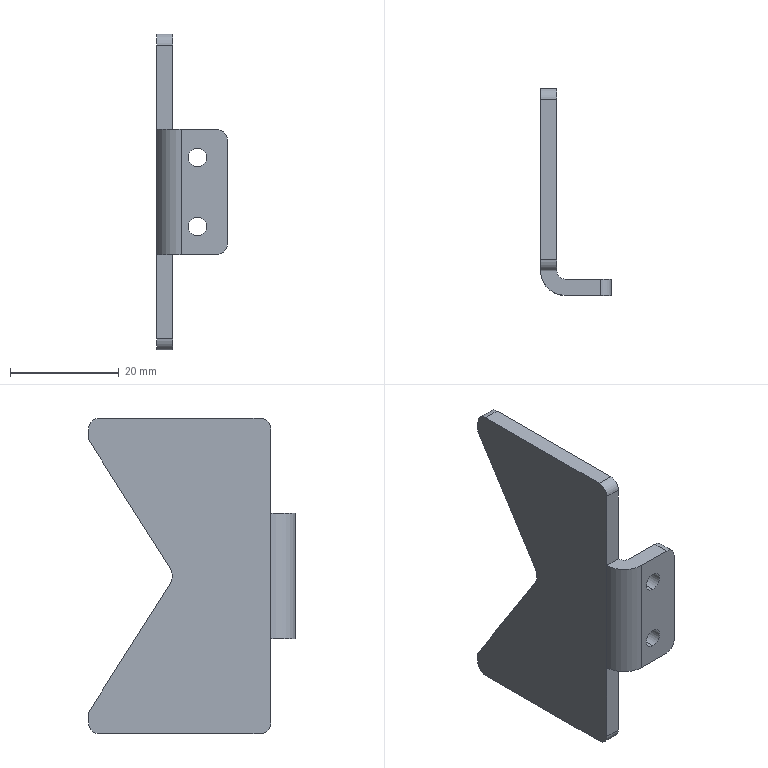Part | SolidWorks | features Fillet 2, ICE 2, FlatPattern 1, HoleWzd 1, SMBaseFlange 1, SheetMetal 1 | 1 solid | 29 faces | box 13 x 38 x 58 mm | volume 5478 mm3 | plane 16 | cylinder 13 | commonest cylinder face diameters 4 x6 3.4 x4 3 x1 6 x1 9 x1
STEP:
#1=CARTESIAN_POINT('',(4.5,-3.,-8.05));
#2=VERTEX_POINT('',#1);
#3=CARTESIAN_POINT('',(4.5,-3.,-4.65));
#4=VERTEX_POINT('',#3);
#5=CARTESIAN_POINT('',(4.5,-3.,-6.35));
#6=DIRECTION('',(0.,1.,0.));
#7=DIRECTION('',(0.,0.,1.));
#8=AXIS2_PLACEMENT_3D('',#5,#6,#7);
#9=CIRCLE('',#8,1.7);
#10=EDGE_CURVE('',#2,#4,#9,.T.);
#11=ORIENTED_EDGE('',*,*,#10,.F.);
#12=CARTESIAN_POINT('',(4.5,0.,-8.05));
#13=VERTEX_POINT('',#12);
#14=CARTESIAN_POINT('',(4.5,0.,-8.05));
#15=DIRECTION('',(0.,1.,0.));
#16=VECTOR('',#15,1000.);
#17=LINE('',#14,#16);
#18=EDGE_CURVE('',#2,#13,#17,.T.);
#19=ORIENTED_EDGE('',*,*,#18,.T.);
#20=CARTESIAN_POINT('',(4.5,0.,-4.65));
#21=VERTEX_POINT('',#20);
#22=CARTESIAN_POINT('',(4.5,0.,-6.35));
#23=DIRECTION('',(0.,1.,0.));
#24=DIRECTION('',(0.,0.,1.));
#25=AXIS2_PLACEMENT_3D('',#22,#23,#24);
#26=CIRCLE('',#25,1.7);
#27=EDGE_CURVE('',#13,#21,#26,.T.);
#28=ORIENTED_EDGE('',*,*,#27,.T.);
#29=CARTESIAN_POINT('',(4.5,0.,-4.65));
#30=DIRECTION('',(0.,1.,0.));
#31=VECTOR('',#30,1000.);
#32=LINE('',#29,#31);
#33=EDGE_CURVE('',#4,#21,#32,.T.);
#34=ORIENTED_EDGE('',*,*,#33,.F.);
#35=EDGE_LOOP('',(#11,#19,#28,#34));
#36=FACE_OUTER_BOUND('',#35,.T.);
#37=CARTESIAN_POINT('',(4.5,0.,-6.35));
#38=DIRECTION('',(0.,1.,0.));
#39=DIRECTION('',(0.,0.,1.));
#40=AXIS2_PLACEMENT_3D('',#37,#38,#39);
#41=CYLINDRICAL_SURFACE('',#40,1.7);
#42=ADVANCED_FACE('',(#36),#41,.F.);
#43=CARTESIAN_POINT('',(4.5,-3.,4.65));
#44=VERTEX_POINT('',#43);
#45=CARTESIAN_POINT('',(4.5,-3.,8.05));
#46=VERTEX_POINT('',#45);
#47=CARTESIAN_POINT('',(4.5,-3.,6.35));
#48=DIRECTION('',(0.,1.,0.));
#49=DIRECTION('',(0.,0.,1.));
#50=AXIS2_PLACEMENT_3D('',#47,#48,#49);
#51=CIRCLE('',#50,1.7);
#52=EDGE_CURVE('',#44,#46,#51,.T.);
#53=ORIENTED_EDGE('',*,*,#52,.F.);
#54=CARTESIAN_POINT('',(4.5,0.,4.65));
#55=VERTEX_POINT('',#54);
#56=CARTESIAN_POINT('',(4.5,0.,4.65));
#57=DIRECTION('',(0.,1.,0.));
#58=VECTOR('',#57,1000.);
#59=LINE('',#56,#58);
#60=EDGE_CURVE('',#44,#55,#59,.T.);
#61=ORIENTED_EDGE('',*,*,#60,.T.);
#62=CARTESIAN_POINT('',(4.5,0.,8.05));
#63=VERTEX_POINT('',#62);
#64=CARTESIAN_POINT('',(4.5,0.,6.35));
#65=DIRECTION('',(0.,1.,0.));
#66=DIRECTION('',(0.,0.,1.));
#67=AXIS2_PLACEMENT_3D('',#64,#65,#66);
#68=CIRCLE('',#67,1.7);
#69=EDGE_CURVE('',#55,#63,#68,.T.);
#70=ORIENTED_EDGE('',*,*,#69,.T.);
#71=CARTESIAN_POINT('',(4.5,0.,8.05));
#72=DIRECTION('',(0.,1.,0.));
#73=VECTOR('',#72,1000.);
#74=LINE('',#71,#73);
#75=EDGE_CURVE('',#46,#63,#74,.T.);
#76=ORIENTED_EDGE('',*,*,#75,.F.);
#77=EDGE_LOOP('',(#53,#61,#70,#76));
#78=FACE_OUTER_BOUND('',#77,.T.);
#79=CARTESIAN_POINT('',(4.5,0.,6.35));
#80=DIRECTION('',(0.,1.,0.));
#81=DIRECTION('',(0.,0.,1.));
#82=AXIS2_PLACEMENT_3D('',#79,#80,#81);
#83=CYLINDRICAL_SURFACE('',#82,1.7);
#84=ADVANCED_FACE('',(#78),#83,.F.);
#85=CARTESIAN_POINT('',(8.,0.,-11.5));
#86=VERTEX_POINT('',#85);
#87=CARTESIAN_POINT('',(1.5,0.,-11.5));
#88=VERTEX_POINT('',#87);
#89=CARTESIAN_POINT('',(0.,0.,-11.5));
#90=DIRECTION('',(-1.,0.,0.));
#91=VECTOR('',#90,1000.);
#92=LINE('',#89,#91);
#93=EDGE_CURVE('',#86,#88,#92,.T.);
#94=ORIENTED_EDGE('',*,*,#93,.F.);
#95=CARTESIAN_POINT('',(8.,-3.,-11.5));
#96=VERTEX_POINT('',#95);
#97=CARTESIAN_POINT('',(8.,1.5,-11.5));
#98=DIRECTION('',(0.,-1.,0.));
#99=VECTOR('',#98,1000.);
#100=LINE('',#97,#99);
#101=EDGE_CURVE('',#86,#96,#100,.T.);
#102=ORIENTED_EDGE('',*,*,#101,.T.);
#103=CARTESIAN_POINT('',(1.5,-3.,-11.5));
#104=VERTEX_POINT('',#103);
#105=CARTESIAN_POINT('',(-3.,-3.,-11.5));
#106=DIRECTION('',(1.,0.,0.));
#107=VECTOR('',#106,1000.);
#108=LINE('',#105,#107);
#109=EDGE_CURVE('',#104,#96,#108,.T.);
#110=ORIENTED_EDGE('',*,*,#109,.F.);
#111=CARTESIAN_POINT('',(1.5,-3.,-11.5));
#112=DIRECTION('',(0.,1.,0.));
#113=VECTOR('',#112,1000.);
#114=LINE('',#111,#113);
#115=EDGE_CURVE('',#104,#88,#114,.T.);
#116=ORIENTED_EDGE('',*,*,#115,.T.);
#117=EDGE_LOOP('',(#94,#102,#110,#116));
#118=FACE_OUTER_BOUND('',#117,.T.);
#119=CARTESIAN_POINT('',(-3.,1.5,-11.5));
#120=DIRECTION('',(0.,0.,1.));
#121=DIRECTION('',(0.,-1.,0.));
#122=AXIS2_PLACEMENT_3D('',#119,#120,#121);
#123=PLANE('',#122);
#124=ADVANCED_FACE('',(#118),#123,.F.);
#125=CARTESIAN_POINT('',(-3.,35.,-27.));
#126=VERTEX_POINT('',#125);
#127=CARTESIAN_POINT('',(-3.,35.,-25.));
#128=VERTEX_POINT('',#127);
#129=CARTESIAN_POINT('',(-3.,35.,-29.));
#130=DIRECTION('',(0.,0.,1.));
#131=VECTOR('',#130,1000.);
#132=LINE('',#129,#131);
#133=EDGE_CURVE('',#126,#128,#132,.T.);
#134=ORIENTED_EDGE('',*,*,#133,.T.);
#135=CARTESIAN_POINT('',(0.,35.,-25.));
#136=VERTEX_POINT('',#135);
#137=CARTESIAN_POINT('',(-3.,35.,-25.));
#138=DIRECTION('',(1.,0.,0.));
#139=VECTOR('',#138,1000.);
#140=LINE('',#137,#139);
#141=EDGE_CURVE('',#128,#136,#140,.T.);
#142=ORIENTED_EDGE('',*,*,#141,.T.);
#143=CARTESIAN_POINT('',(0.,35.,-27.));
#144=VERTEX_POINT('',#143);
#145=CARTESIAN_POINT('',(0.,35.,-29.));
#146=DIRECTION('',(0.,0.,1.));
#147=VECTOR('',#146,1000.);
#148=LINE('',#145,#147);
#149=EDGE_CURVE('',#144,#136,#148,.T.);
#150=ORIENTED_EDGE('',*,*,#149,.F.);
#151=CARTESIAN_POINT('',(-3.,35.,-27.));
#152=DIRECTION('',(-1.,0.,0.));
#153=VECTOR('',#152,1000.);
#154=LINE('',#151,#153);
#155=EDGE_CURVE('',#144,#126,#154,.T.);
#156=ORIENTED_EDGE('',*,*,#155,.T.);
#157=EDGE_LOOP('',(#134,#142,#150,#156));
#158=FACE_OUTER_BOUND('',#157,.T.);
#159=CARTESIAN_POINT('',(-3.,35.,-29.));
#160=DIRECTION('',(0.,-1.,0.));
#161=DIRECTION('',(0.,0.,-1.));
#162=AXIS2_PLACEMENT_3D('',#159,#160,#161);
#163=PLANE('',#162);
#164=ADVANCED_FACE('',(#158),#163,.F.);
#165=CARTESIAN_POINT('',(0.,33.,-29.));
#166=VERTEX_POINT('',#165);
#167=CARTESIAN_POINT('',(0.,3.5,-29.));
#168=VERTEX_POINT('',#167);
#169=CARTESIAN_POINT('',(0.,35.,-29.));
#170=DIRECTION('',(0.,-1.,0.));
#171=VECTOR('',#170,1000.);
#172=LINE('',#169,#171);
#173=EDGE_CURVE('',#166,#168,#172,.T.);
#174=ORIENTED_EDGE('',*,*,#173,.T.);
#175=CARTESIAN_POINT('',(-3.,3.5,-29.));
#176=VERTEX_POINT('',#175);
#177=CARTESIAN_POINT('',(-3.,3.5,-29.));
#178=DIRECTION('',(-1.,0.,0.));
#179=VECTOR('',#178,1000.);
#180=LINE('',#177,#179);
#181=EDGE_CURVE('',#168,#176,#180,.T.);
#182=ORIENTED_EDGE('',*,*,#181,.T.);
#183=CARTESIAN_POINT('',(-3.,33.,-29.));
#184=VERTEX_POINT('',#183);
#185=CARTESIAN_POINT('',(-3.,35.,-29.));
#186=DIRECTION('',(0.,-1.,0.));
#187=VECTOR('',#186,1000.);
#188=LINE('',#185,#187);
#189=EDGE_CURVE('',#184,#176,#188,.T.);
#190=ORIENTED_EDGE('',*,*,#189,.F.);
#191=CARTESIAN_POINT('',(0.,33.,-29.));
#192=DIRECTION('',(1.,0.,0.));
#193=VECTOR('',#192,1000.);
#194=LINE('',#191,#193);
#195=EDGE_CURVE('',#184,#166,#194,.T.);
#196=ORIENTED_EDGE('',*,*,#195,.T.);
#197=EDGE_LOOP('',(#174,#182,#190,#196));
#198=FACE_OUTER_BOUND('',#197,.T.);
#199=CARTESIAN_POINT('',(1.5,-3.,-29.));
#200=DIRECTION('',(0.,0.,-1.));
#201=DIRECTION('',(-1.,0.,0.));
#202=AXIS2_PLACEMENT_3D('',#199,#200,#201);
#203=PLANE('',#202);
#204=ADVANCED_FACE('',(#198),#203,.T.);
#205=ORIENTED_EDGE('',*,*,#109,.T.);
#206=CARTESIAN_POINT('',(10.,-3.,-9.5));
#207=VERTEX_POINT('',#206);
#208=CARTESIAN_POINT('',(8.,-3.,-9.5));
#209=DIRECTION('',(0.,-1.,0.));
#210=DIRECTION('',(0.,0.,-1.));
#211=AXIS2_PLACEMENT_3D('',#208,#209,#210);
#212=CIRCLE('',#211,2.);
#213=EDGE_CURVE('',#96,#207,#212,.T.);
#214=ORIENTED_EDGE('',*,*,#213,.T.);
#215=CARTESIAN_POINT('',(10.,-3.,9.5));
#216=VERTEX_POINT('',#215);
#217=CARTESIAN_POINT('',(10.,-3.,-29.));
#218=DIRECTION('',(0.,0.,1.));
#219=VECTOR('',#218,1000.);
#220=LINE('',#217,#219);
#221=EDGE_CURVE('',#207,#216,#220,.T.);
#222=ORIENTED_EDGE('',*,*,#221,.T.);
#223=CARTESIAN_POINT('',(8.,-3.,11.5));
#224=VERTEX_POINT('',#223);
#225=CARTESIAN_POINT('',(8.,-3.,9.5));
#226=DIRECTION('',(0.,-1.,0.));
#227=DIRECTION('',(0.,0.,-1.));
#228=AXIS2_PLACEMENT_3D('',#225,#226,#227);
#229=CIRCLE('',#228,2.);
#230=EDGE_CURVE('',#216,#224,#229,.T.);
#231=ORIENTED_EDGE('',*,*,#230,.T.);
#232=CARTESIAN_POINT('',(1.5,-3.,11.5));
#233=VERTEX_POINT('',#232);
#234=CARTESIAN_POINT('',(-3.,-3.,11.5));
#235=DIRECTION('',(1.,0.,0.));
#236=VECTOR('',#235,1000.);
#237=LINE('',#234,#236);
#238=EDGE_CURVE('',#233,#224,#237,.T.);
#239=ORIENTED_EDGE('',*,*,#238,.F.);
#240=CARTESIAN_POINT('',(1.5,-3.,-29.));
#241=DIRECTION('',(0.,0.,1.));
#242=VECTOR('',#241,1000.);
#243=LINE('',#240,#242);
#244=EDGE_CURVE('',#104,#233,#243,.T.);
#245=ORIENTED_EDGE('',*,*,#244,.F.);
#246=EDGE_LOOP('',(#205,#214,#222,#231,#239,#245));
#247=FACE_OUTER_BOUND('',#246,.T.);
#248=CARTESIAN_POINT('',(4.5,-3.,-6.35));
#249=DIRECTION('',(0.,1.,0.));
#250=DIRECTION('',(0.,0.,1.));
#251=AXIS2_PLACEMENT_3D('',#248,#249,#250);
#252=CIRCLE('',#251,1.7);
#253=EDGE_CURVE('',#4,#2,#252,.T.);
#254=ORIENTED_EDGE('',*,*,#253,.T.);
#255=ORIENTED_EDGE('',*,*,#10,.T.);
#256=EDGE_LOOP('',(#254,#255));
#257=FACE_BOUND('',#256,.T.);
#258=CARTESIAN_POINT('',(4.5,-3.,6.35));
#259=DIRECTION('',(0.,1.,0.));
#260=DIRECTION('',(0.,0.,1.));
#261=AXIS2_PLACEMENT_3D('',#258,#259,#260);
#262=CIRCLE('',#261,1.7);
#263=EDGE_CURVE('',#46,#44,#262,.T.);
#264=ORIENTED_EDGE('',*,*,#263,.T.);
#265=ORIENTED_EDGE('',*,*,#52,.T.);
#266=EDGE_LOOP('',(#264,#265));
#267=FACE_BOUND('',#266,.T.);
#268=CARTESIAN_POINT('',(0.,-3.,-29.));
#269=DIRECTION('',(0.,-1.,0.));
#270=DIRECTION('',(0.,0.,-1.));
#271=AXIS2_PLACEMENT_3D('',#268,#269,#270);
#272=PLANE('',#271);
#273=ADVANCED_FACE('',(#247,#257,#267),#272,.T.);
#274=CARTESIAN_POINT('',(-3.,1.5,11.5));
#275=VERTEX_POINT('',#274);
#276=CARTESIAN_POINT('',(1.5,1.5,11.5));
#277=DIRECTION('',(0.,0.,1.));
#278=DIRECTION('',(0.,1.,0.));
#279=AXIS2_PLACEMENT_3D('',#276,#277,#278);
#280=CIRCLE('',#279,4.5);
#281=EDGE_CURVE('',#275,#233,#280,.T.);
#282=ORIENTED_EDGE('',*,*,#281,.F.);
#283=CARTESIAN_POINT('',(-3.,1.5,-11.5));
#284=VERTEX_POINT('',#283);
#285=CARTESIAN_POINT('',(-3.,1.5,-29.));
#286=DIRECTION('',(0.,0.,1.));
#287=VECTOR('',#286,1000.);
#288=LINE('',#285,#287);
#289=EDGE_CURVE('',#284,#275,#288,.T.);
#290=ORIENTED_EDGE('',*,*,#289,.F.);
#291=CARTESIAN_POINT('',(1.5,1.5,-11.5));
#292=DIRECTION('',(0.,0.,-1.));
#293=DIRECTION('',(0.,-1.,0.));
#294=AXIS2_PLACEMENT_3D('',#291,#292,#293);
#295=CIRCLE('',#294,4.5);
#296=EDGE_CURVE('',#104,#284,#295,.T.);
#297=ORIENTED_EDGE('',*,*,#296,.F.);
#298=ORIENTED_EDGE('',*,*,#244,.T.);
#299=EDGE_LOOP('',(#282,#290,#297,#298));
#300=FACE_OUTER_BOUND('',#299,.T.);
#301=CARTESIAN_POINT('',(1.5,1.5,-29.));
#302=DIRECTION('',(0.,0.,1.));
#303=DIRECTION('',(1.,0.,0.));
#304=AXIS2_PLACEMENT_3D('',#301,#302,#303);
#305=CYLINDRICAL_SURFACE('',#304,4.5);
#306=ADVANCED_FACE('',(#300),#305,.T.);
#307=ORIENTED_EDGE('',*,*,#189,.T.);
#308=CARTESIAN_POINT('',(-3.,1.5,-27.));
#309=VERTEX_POINT('',#308);
#310=CARTESIAN_POINT('',(-3.,3.5,-27.));
#311=DIRECTION('',(-1.,0.,0.));
#312=DIRECTION('',(0.,-1.,0.));
#313=AXIS2_PLACEMENT_3D('',#310,#311,#312);
#314=CIRCLE('',#313,2.);
#315=EDGE_CURVE('',#176,#309,#314,.T.);
#316=ORIENTED_EDGE('',*,*,#315,.T.);
#317=CARTESIAN_POINT('',(-3.,1.5,-29.));
#318=DIRECTION('',(0.,0.,1.));
#319=VECTOR('',#318,1000.);
#320=LINE('',#317,#319);
#321=EDGE_CURVE('',#309,#284,#320,.T.);
#322=ORIENTED_EDGE('',*,*,#321,.T.);
#323=ORIENTED_EDGE('',*,*,#289,.T.);
#324=CARTESIAN_POINT('',(-3.,1.5,27.));
#325=VERTEX_POINT('',#324);
#326=CARTESIAN_POINT('',(-3.,1.5,29.));
#327=DIRECTION('',(0.,0.,1.));
#328=VECTOR('',#327,1000.);
#329=LINE('',#326,#328);
#330=EDGE_CURVE('',#275,#325,#329,.T.);
#331=ORIENTED_EDGE('',*,*,#330,.T.);
#332=CARTESIAN_POINT('',(-3.,3.5,29.));
#333=VERTEX_POINT('',#332);
#334=CARTESIAN_POINT('',(-3.,3.5,27.));
#335=DIRECTION('',(-1.,0.,0.));
#336=DIRECTION('',(0.,-1.,0.));
#337=AXIS2_PLACEMENT_3D('',#334,#335,#336);
#338=CIRCLE('',#337,2.);
#339=EDGE_CURVE('',#325,#333,#338,.T.);
#340=ORIENTED_EDGE('',*,*,#339,.T.);
#341=CARTESIAN_POINT('',(-3.,33.,29.));
#342=VERTEX_POINT('',#341);
#343=CARTESIAN_POINT('',(-3.,35.,29.));
#344=DIRECTION('',(0.,-1.,0.));
#345=VECTOR('',#344,1000.);
#346=LINE('',#343,#345);
#347=EDGE_CURVE('',#342,#333,#346,.T.);
#348=ORIENTED_EDGE('',*,*,#347,.F.);
#349=CARTESIAN_POINT('',(-3.,35.,27.));
#350=VERTEX_POINT('',#349);
#351=CARTESIAN_POINT('',(-3.,33.,27.));
#352=DIRECTION('',(-1.,0.,0.));
#353=DIRECTION('',(0.,-1.,0.));
#354=AXIS2_PLACEMENT_3D('',#351,#352,#353);
#355=CIRCLE('',#354,2.);
#356=EDGE_CURVE('',#342,#350,#355,.T.);
#357=ORIENTED_EDGE('',*,*,#356,.T.);
#358=CARTESIAN_POINT('',(-3.,35.,25.));
#359=VERTEX_POINT('',#358);
#360=CARTESIAN_POINT('',(-3.,35.,-29.));
#361=DIRECTION('',(0.,0.,1.));
#362=VECTOR('',#361,1000.);
#363=LINE('',#360,#362);
#364=EDGE_CURVE('',#359,#350,#363,.T.);
#365=ORIENTED_EDGE('',*,*,#364,.F.);
#366=CARTESIAN_POINT('',(-3.,20.1,1.612));
#367=VERTEX_POINT('',#366);
#368=CARTESIAN_POINT('',(-3.,35.,25.));
#369=DIRECTION('',(0.,-0.5373,-0.8434));
#370=VECTOR('',#369,1000.);
#371=LINE('',#368,#370);
#372=EDGE_CURVE('',#359,#367,#371,.T.);
#373=ORIENTED_EDGE('',*,*,#372,.T.);
#374=CARTESIAN_POINT('',(-3.,20.1,-1.612));
#375=VERTEX_POINT('',#374);
#376=CARTESIAN_POINT('',(-3.,22.63,0.));
#377=DIRECTION('',(1.,0.,0.));
#378=DIRECTION('',(0.,1.,0.));
#379=AXIS2_PLACEMENT_3D('',#376,#377,#378);
#380=CIRCLE('',#379,3.);
#381=EDGE_CURVE('',#367,#375,#380,.T.);
#382=ORIENTED_EDGE('',*,*,#381,.T.);
#383=CARTESIAN_POINT('',(-3.,35.,-25.));
#384=DIRECTION('',(0.,0.5373,-0.8434));
#385=VECTOR('',#384,1000.);
#386=LINE('',#383,#385);
#387=EDGE_CURVE('',#375,#128,#386,.T.);
#388=ORIENTED_EDGE('',*,*,#387,.T.);
#389=ORIENTED_EDGE('',*,*,#133,.F.);
#390=CARTESIAN_POINT('',(-3.,33.,-27.));
#391=DIRECTION('',(-1.,0.,0.));
#392=DIRECTION('',(0.,-1.,0.));
#393=AXIS2_PLACEMENT_3D('',#390,#391,#392);
#394=CIRCLE('',#393,2.);
#395=EDGE_CURVE('',#126,#184,#394,.T.);
#396=ORIENTED_EDGE('',*,*,#395,.T.);
#397=EDGE_LOOP('',(#307,#316,#322,#323,#331,#340,#348,#357,#365,#373,#382,#388,#389,#396));
#398=FACE_OUTER_BOUND('',#397,.T.);
#399=CARTESIAN_POINT('',(-3.,35.,-29.));
#400=DIRECTION('',(-1.,0.,0.));
#401=DIRECTION('',(0.,-1.,0.));
#402=AXIS2_PLACEMENT_3D('',#399,#400,#401);
#403=PLANE('',#402);
#404=ADVANCED_FACE('',(#398),#403,.T.);
#405=CARTESIAN_POINT('',(0.,35.,25.));
#406=VERTEX_POINT('',#405);
#407=CARTESIAN_POINT('',(0.,35.,27.));
#408=VERTEX_POINT('',#407);
#409=CARTESIAN_POINT('',(0.,35.,-29.));
#410=DIRECTION('',(0.,0.,1.));
#411=VECTOR('',#410,1000.);
#412=LINE('',#409,#411);
#413=EDGE_CURVE('',#406,#408,#412,.T.);
#414=ORIENTED_EDGE('',*,*,#413,.F.);
#415=CARTESIAN_POINT('',(-3.,35.,25.));
#416=DIRECTION('',(1.,0.,0.));
#417=VECTOR('',#416,1000.);
#418=LINE('',#415,#417);
#419=EDGE_CURVE('',#359,#406,#418,.T.);
#420=ORIENTED_EDGE('',*,*,#419,.F.);
#421=ORIENTED_EDGE('',*,*,#364,.T.);
#422=CARTESIAN_POINT('',(-3.,35.,27.));
#423=DIRECTION('',(1.,0.,0.));
#424=VECTOR('',#423,1000.);
#425=LINE('',#422,#424);
#426=EDGE_CURVE('',#350,#408,#425,.T.);
#427=ORIENTED_EDGE('',*,*,#426,.T.);
#428=EDGE_LOOP('',(#414,#420,#421,#427));
#429=FACE_OUTER_BOUND('',#428,.T.);
#430=CARTESIAN_POINT('',(-3.,35.,-29.));
#431=DIRECTION('',(0.,-1.,0.));
#432=DIRECTION('',(0.,0.,-1.));
#433=AXIS2_PLACEMENT_3D('',#430,#431,#432);
#434=PLANE('',#433);
#435=ADVANCED_FACE('',(#429),#434,.F.);
#436=CARTESIAN_POINT('',(0.,1.5,-27.));
#437=VERTEX_POINT('',#436);
#438=CARTESIAN_POINT('',(0.,1.5,-11.5));
#439=VERTEX_POINT('',#438);
#440=CARTESIAN_POINT('',(0.,1.5,-29.));
#441=DIRECTION('',(0.,0.,1.));
#442=VECTOR('',#441,1000.);
#443=LINE('',#440,#442);
#444=EDGE_CURVE('',#437,#439,#443,.T.);
#445=ORIENTED_EDGE('',*,*,#444,.F.);
#446=CARTESIAN_POINT('',(0.,3.5,-27.));
#447=DIRECTION('',(1.,0.,0.));
#448=DIRECTION('',(0.,-1.,0.));
#449=AXIS2_PLACEMENT_3D('',#446,#447,#448);
#450=CIRCLE('',#449,2.);
#451=EDGE_CURVE('',#437,#168,#450,.T.);
#452=ORIENTED_EDGE('',*,*,#451,.T.);
#453=ORIENTED_EDGE('',*,*,#173,.F.);
#454=CARTESIAN_POINT('',(0.,33.,-27.));
#455=DIRECTION('',(1.,0.,0.));
#456=DIRECTION('',(0.,-1.,0.));
#457=AXIS2_PLACEMENT_3D('',#454,#455,#456);
#458=CIRCLE('',#457,2.);
#459=EDGE_CURVE('',#166,#144,#458,.T.);
#460=ORIENTED_EDGE('',*,*,#459,.T.);
#461=ORIENTED_EDGE('',*,*,#149,.T.);
#462=CARTESIAN_POINT('',(0.,20.1,-1.612));
#463=VERTEX_POINT('',#462);
#464=CARTESIAN_POINT('',(0.,35.,-25.));
#465=DIRECTION('',(0.,0.5373,-0.8434));
#466=VECTOR('',#465,1000.);
#467=LINE('',#464,#466);
#468=EDGE_CURVE('',#463,#136,#467,.T.);
#469=ORIENTED_EDGE('',*,*,#468,.F.);
#470=CARTESIAN_POINT('',(0.,20.1,1.612));
#471=VERTEX_POINT('',#470);
#472=CARTESIAN_POINT('',(0.,22.63,0.));
#473=DIRECTION('',(1.,0.,0.));
#474=DIRECTION('',(0.,1.,0.));
#475=AXIS2_PLACEMENT_3D('',#472,#473,#474);
#476=CIRCLE('',#475,3.);
#477=EDGE_CURVE('',#471,#463,#476,.T.);
#478=ORIENTED_EDGE('',*,*,#477,.F.);
#479=CARTESIAN_POINT('',(0.,35.,25.));
#480=DIRECTION('',(0.,-0.5373,-0.8434));
#481=VECTOR('',#480,1000.);
#482=LINE('',#479,#481);
#483=EDGE_CURVE('',#406,#471,#482,.T.);
#484=ORIENTED_EDGE('',*,*,#483,.F.);
#485=ORIENTED_EDGE('',*,*,#413,.T.);
#486=CARTESIAN_POINT('',(0.,33.,29.));
#487=VERTEX_POINT('',#486);
#488=CARTESIAN_POINT('',(0.,33.,27.));
#489=DIRECTION('',(1.,0.,0.));
#490=DIRECTION('',(0.,-1.,0.));
#491=AXIS2_PLACEMENT_3D('',#488,#489,#490);
#492=CIRCLE('',#491,2.);
#493=EDGE_CURVE('',#408,#487,#492,.T.);
#494=ORIENTED_EDGE('',*,*,#493,.T.);
#495=CARTESIAN_POINT('',(0.,3.5,29.));
#496=VERTEX_POINT('',#495);
#497=CARTESIAN_POINT('',(0.,35.,29.));
#498=DIRECTION('',(0.,-1.,0.));
#499=VECTOR('',#498,1000.);
#500=LINE('',#497,#499);
#501=EDGE_CURVE('',#487,#496,#500,.T.);
#502=ORIENTED_EDGE('',*,*,#501,.T.);
#503=CARTESIAN_POINT('',(0.,1.5,27.));
#504=VERTEX_POINT('',#503);
#505=CARTESIAN_POINT('',(0.,3.5,27.));
#506=DIRECTION('',(1.,0.,0.));
#507=DIRECTION('',(0.,-1.,0.));
#508=AXIS2_PLACEMENT_3D('',#505,#506,#507);
#509=CIRCLE('',#508,2.);
#510=EDGE_CURVE('',#496,#504,#509,.T.);
#511=ORIENTED_EDGE('',*,*,#510,.T.);
#512=CARTESIAN_POINT('',(0.,1.5,11.5));
#513=VERTEX_POINT('',#512);
#514=CARTESIAN_POINT('',(0.,1.5,-29.));
#515=DIRECTION('',(0.,0.,-1.));
#516=VECTOR('',#515,1000.);
#517=LINE('',#514,#516);
#518=EDGE_CURVE('',#504,#513,#517,.T.);
#519=ORIENTED_EDGE('',*,*,#518,.T.);
#520=CARTESIAN_POINT('',(0.,1.5,-29.));
#521=DIRECTION('',(0.,0.,1.));
#522=VECTOR('',#521,1000.);
#523=LINE('',#520,#522);
#524=EDGE_CURVE('',#439,#513,#523,.T.);
#525=ORIENTED_EDGE('',*,*,#524,.F.);
#526=EDGE_LOOP('',(#445,#452,#453,#460,#461,#469,#478,#484,#485,#494,#502,#511,#519,#525));
#527=FACE_OUTER_BOUND('',#526,.T.);
#528=CARTESIAN_POINT('',(0.,35.,-29.));
#529=DIRECTION('',(-1.,0.,0.));
#530=DIRECTION('',(0.,-1.,0.));
#531=AXIS2_PLACEMENT_3D('',#528,#529,#530);
#532=PLANE('',#531);
#533=ADVANCED_FACE('',(#527),#532,.F.);
#534=ORIENTED_EDGE('',*,*,#524,.T.);
#535=CARTESIAN_POINT('',(1.5,0.,11.5));
#536=VERTEX_POINT('',#535);
#537=CARTESIAN_POINT('',(1.5,1.5,11.5));
#538=DIRECTION('',(0.,0.,1.));
#539=DIRECTION('',(0.,1.,0.));
#540=AXIS2_PLACEMENT_3D('',#537,#538,#539);
#541=CIRCLE('',#540,1.5);
#542=EDGE_CURVE('',#513,#536,#541,.T.);
#543=ORIENTED_EDGE('',*,*,#542,.T.);
#544=CARTESIAN_POINT('',(1.5,0.,-29.));
#545=DIRECTION('',(0.,0.,1.));
#546=VECTOR('',#545,1000.);
#547=LINE('',#544,#546);
#548=EDGE_CURVE('',#88,#536,#547,.T.);
#549=ORIENTED_EDGE('',*,*,#548,.F.);
#550=CARTESIAN_POINT('',(1.5,1.5,-11.5));
#551=DIRECTION('',(0.,0.,-1.));
#552=DIRECTION('',(0.,-1.,0.));
#553=AXIS2_PLACEMENT_3D('',#550,#551,#552);
#554=CIRCLE('',#553,1.5);
#555=EDGE_CURVE('',#88,#439,#554,.T.);
#556=ORIENTED_EDGE('',*,*,#555,.T.);
#557=EDGE_LOOP('',(#534,#543,#549,#556));
#558=FACE_OUTER_BOUND('',#557,.T.);
#559=CARTESIAN_POINT('',(1.5,1.5,-29.));
#560=DIRECTION('',(0.,0.,1.));
#561=DIRECTION('',(1.,0.,0.));
#562=AXIS2_PLACEMENT_3D('',#559,#560,#561);
#563=CYLINDRICAL_SURFACE('',#562,1.5);
#564=ADVANCED_FACE('',(#558),#563,.F.);
#565=CARTESIAN_POINT('',(4.5,0.,-6.35));
#566=DIRECTION('',(0.,1.,0.));
#567=DIRECTION('',(0.,0.,1.));
#568=AXIS2_PLACEMENT_3D('',#565,#566,#567);
#569=CIRCLE('',#568,1.7);
#570=EDGE_CURVE('',#21,#13,#569,.T.);
#571=ORIENTED_EDGE('',*,*,#570,.F.);
#572=ORIENTED_EDGE('',*,*,#27,.F.);
#573=EDGE_LOOP('',(#571,#572));
#574=FACE_BOUND('',#573,.T.);
#575=CARTESIAN_POINT('',(4.5,0.,6.35));
#576=DIRECTION('',(0.,1.,0.));
#577=DIRECTION('',(0.,0.,1.));
#578=AXIS2_PLACEMENT_3D('',#575,#576,#577);
#579=CIRCLE('',#578,1.7);
#580=EDGE_CURVE('',#63,#55,#579,.T.);
#581=ORIENTED_EDGE('',*,*,#580,.F.);
#582=ORIENTED_EDGE('',*,*,#69,.F.);
#583=EDGE_LOOP('',(#581,#582));
#584=FACE_BOUND('',#583,.T.);
#585=CARTESIAN_POINT('',(10.,0.,-9.5));
#586=VERTEX_POINT('',#585);
#587=CARTESIAN_POINT('',(10.,0.,9.5));
#588=VERTEX_POINT('',#587);
#589=CARTESIAN_POINT('',(10.,0.,-29.));
#590=DIRECTION('',(0.,0.,1.));
#591=VECTOR('',#590,1000.);
#592=LINE('',#589,#591);
#593=EDGE_CURVE('',#586,#588,#592,.T.);
#594=ORIENTED_EDGE('',*,*,#593,.F.);
#595=CARTESIAN_POINT('',(8.,0.,-9.5));
#596=DIRECTION('',(0.,1.,0.));
#597=DIRECTION('',(0.,0.,-1.));
#598=AXIS2_PLACEMENT_3D('',#595,#596,#597);
#599=CIRCLE('',#598,2.);
#600=EDGE_CURVE('',#586,#86,#599,.T.);
#601=ORIENTED_EDGE('',*,*,#600,.T.);
#602=ORIENTED_EDGE('',*,*,#93,.T.);
#603=ORIENTED_EDGE('',*,*,#548,.T.);
#604=CARTESIAN_POINT('',(8.,0.,11.5));
#605=VERTEX_POINT('',#604);
#606=CARTESIAN_POINT('',(0.,0.,11.5));
#607=DIRECTION('',(1.,0.,0.));
#608=VECTOR('',#607,1000.);
#609=LINE('',#606,#608);
#610=EDGE_CURVE('',#536,#605,#609,.T.);
#611=ORIENTED_EDGE('',*,*,#610,.T.);
#612=CARTESIAN_POINT('',(8.,0.,9.5));
#613=DIRECTION('',(0.,1.,0.));
#614=DIRECTION('',(0.,0.,-1.));
#615=AXIS2_PLACEMENT_3D('',#612,#613,#614);
#616=CIRCLE('',#615,2.);
#617=EDGE_CURVE('',#605,#588,#616,.T.);
#618=ORIENTED_EDGE('',*,*,#617,.T.);
#619=EDGE_LOOP('',(#594,#601,#602,#603,#611,#618));
#620=FACE_OUTER_BOUND('',#619,.T.);
#621=CARTESIAN_POINT('',(0.,0.,-29.));
#622=DIRECTION('',(0.,-1.,0.));
#623=DIRECTION('',(0.,0.,-1.));
#624=AXIS2_PLACEMENT_3D('',#621,#622,#623);
#625=PLANE('',#624);
#626=ADVANCED_FACE('',(#574,#584,#620),#625,.F.);
#627=ORIENTED_EDGE('',*,*,#221,.F.);
#628=CARTESIAN_POINT('',(10.,0.,-9.5));
#629=DIRECTION('',(0.,1.,0.));
#630=VECTOR('',#629,1000.);
#631=LINE('',#628,#630);
#632=EDGE_CURVE('',#207,#586,#631,.T.);
#633=ORIENTED_EDGE('',*,*,#632,.T.);
#634=ORIENTED_EDGE('',*,*,#593,.T.);
#635=CARTESIAN_POINT('',(10.,0.,9.5));
#636=DIRECTION('',(0.,-1.,0.));
#637=VECTOR('',#636,1000.);
#638=LINE('',#635,#637);
#639=EDGE_CURVE('',#588,#216,#638,.T.);
#640=ORIENTED_EDGE('',*,*,#639,.T.);
#641=EDGE_LOOP('',(#627,#633,#634,#640));
#642=FACE_OUTER_BOUND('',#641,.T.);
#643=CARTESIAN_POINT('',(10.,0.,-29.));
#644=DIRECTION('',(-1.,0.,0.));
#645=DIRECTION('',(0.,0.,1.));
#646=AXIS2_PLACEMENT_3D('',#643,#644,#645);
#647=PLANE('',#646);
#648=ADVANCED_FACE('',(#642),#647,.F.);
#649=ORIENTED_EDGE('',*,*,#347,.T.);
#650=CARTESIAN_POINT('',(1.5,3.5,29.));
#651=DIRECTION('',(1.,0.,0.));
#652=VECTOR('',#651,1000.);
#653=LINE('',#650,#652);
#654=EDGE_CURVE('',#333,#496,#653,.T.);
#655=ORIENTED_EDGE('',*,*,#654,.T.);
#656=ORIENTED_EDGE('',*,*,#501,.F.);
#657=CARTESIAN_POINT('',(1.5,33.,29.));
#658=DIRECTION('',(-1.,0.,0.));
#659=VECTOR('',#658,1000.);
#660=LINE('',#657,#659);
#661=EDGE_CURVE('',#487,#342,#660,.T.);
#662=ORIENTED_EDGE('',*,*,#661,.T.);
#663=EDGE_LOOP('',(#649,#655,#656,#662));
#664=FACE_OUTER_BOUND('',#663,.T.);
#665=CARTESIAN_POINT('',(1.5,1.5,29.));
#666=DIRECTION('',(0.,0.,-1.));
#667=DIRECTION('',(-1.,0.,0.));
#668=AXIS2_PLACEMENT_3D('',#665,#666,#667);
#669=PLANE('',#668);
#670=ADVANCED_FACE('',(#664),#669,.F.);
#671=ORIENTED_EDGE('',*,*,#60,.F.);
#672=ORIENTED_EDGE('',*,*,#263,.F.);
#673=ORIENTED_EDGE('',*,*,#75,.T.);
#674=ORIENTED_EDGE('',*,*,#580,.T.);
#675=EDGE_LOOP('',(#671,#672,#673,#674));
#676=FACE_OUTER_BOUND('',#675,.T.);
#677=CARTESIAN_POINT('',(4.5,0.,6.35));
#678=DIRECTION('',(0.,1.,0.));
#679=DIRECTION('',(0.,0.,1.));
#680=AXIS2_PLACEMENT_3D('',#677,#678,#679);
#681=CYLINDRICAL_SURFACE('',#680,1.7);
#682=ADVANCED_FACE('',(#676),#681,.F.);
#683=ORIENTED_EDGE('',*,*,#18,.F.);
#684=ORIENTED_EDGE('',*,*,#253,.F.);
#685=ORIENTED_EDGE('',*,*,#33,.T.);
#686=ORIENTED_EDGE('',*,*,#570,.T.);
#687=EDGE_LOOP('',(#683,#684,#685,#686));
#688=FACE_OUTER_BOUND('',#687,.T.);
#689=CARTESIAN_POINT('',(4.5,0.,-6.35));
#690=DIRECTION('',(0.,1.,0.));
#691=DIRECTION('',(0.,0.,1.));
#692=AXIS2_PLACEMENT_3D('',#689,#690,#691);
#693=CYLINDRICAL_SURFACE('',#692,1.7);
#694=ADVANCED_FACE('',(#688),#693,.F.);
#695=ORIENTED_EDGE('',*,*,#356,.F.);
#696=ORIENTED_EDGE('',*,*,#661,.F.);
#697=ORIENTED_EDGE('',*,*,#493,.F.);
#698=ORIENTED_EDGE('',*,*,#426,.F.);
#699=EDGE_LOOP('',(#695,#696,#697,#698));
#700=FACE_OUTER_BOUND('',#699,.T.);
#701=CARTESIAN_POINT('',(-3.,33.,27.));
#702=DIRECTION('',(1.,0.,0.));
#703=DIRECTION('',(0.,0.,-1.));
#704=AXIS2_PLACEMENT_3D('',#701,#702,#703);
#705=CYLINDRICAL_SURFACE('',#704,2.);
#706=ADVANCED_FACE('',(#700),#705,.T.);
#707=ORIENTED_EDGE('',*,*,#395,.F.);
#708=ORIENTED_EDGE('',*,*,#155,.F.);
#709=ORIENTED_EDGE('',*,*,#459,.F.);
#710=ORIENTED_EDGE('',*,*,#195,.F.);
#711=EDGE_LOOP('',(#707,#708,#709,#710));
#712=FACE_OUTER_BOUND('',#711,.T.);
#713=CARTESIAN_POINT('',(1.5,33.,-27.));
#714=DIRECTION('',(-1.,0.,0.));
#715=DIRECTION('',(0.,0.,1.));
#716=AXIS2_PLACEMENT_3D('',#713,#714,#715);
#717=CYLINDRICAL_SURFACE('',#716,2.);
#718=ADVANCED_FACE('',(#712),#717,.T.);
#719=ORIENTED_EDGE('',*,*,#468,.T.);
#720=ORIENTED_EDGE('',*,*,#141,.F.);
#721=ORIENTED_EDGE('',*,*,#387,.F.);
#722=CARTESIAN_POINT('',(-3.,20.1,-1.612));
#723=DIRECTION('',(1.,0.,0.));
#724=VECTOR('',#723,1000.);
#725=LINE('',#722,#724);
#726=EDGE_CURVE('',#375,#463,#725,.T.);
#727=ORIENTED_EDGE('',*,*,#726,.T.);
#728=EDGE_LOOP('',(#719,#720,#721,#727));
#729=FACE_OUTER_BOUND('',#728,.T.);
#730=CARTESIAN_POINT('',(-3.,35.,-25.));
#731=DIRECTION('',(0.,-0.8434,-0.5373));
#732=DIRECTION('',(0.,0.5373,-0.8434));
#733=AXIS2_PLACEMENT_3D('',#730,#731,#732);
#734=PLANE('',#733);
#735=ADVANCED_FACE('',(#729),#734,.F.);
#736=ORIENTED_EDGE('',*,*,#477,.T.);
#737=ORIENTED_EDGE('',*,*,#726,.F.);
#738=ORIENTED_EDGE('',*,*,#381,.F.);
#739=CARTESIAN_POINT('',(-3.,20.1,1.612));
#740=DIRECTION('',(1.,0.,0.));
#741=VECTOR('',#740,1000.);
#742=LINE('',#739,#741);
#743=EDGE_CURVE('',#367,#471,#742,.T.);
#744=ORIENTED_EDGE('',*,*,#743,.T.);
#745=EDGE_LOOP('',(#736,#737,#738,#744));
#746=FACE_OUTER_BOUND('',#745,.T.);
#747=CARTESIAN_POINT('',(-3.,22.63,0.));
#748=DIRECTION('',(1.,0.,0.));
#749=DIRECTION('',(0.,1.,0.));
#750=AXIS2_PLACEMENT_3D('',#747,#748,#749);
#751=CYLINDRICAL_SURFACE('',#750,3.);
#752=ADVANCED_FACE('',(#746),#751,.F.);
#753=ORIENTED_EDGE('',*,*,#483,.T.);
#754=ORIENTED_EDGE('',*,*,#743,.F.);
#755=ORIENTED_EDGE('',*,*,#372,.F.);
#756=ORIENTED_EDGE('',*,*,#419,.T.);
#757=EDGE_LOOP('',(#753,#754,#755,#756));
#758=FACE_OUTER_BOUND('',#757,.T.);
#759=CARTESIAN_POINT('',(-3.,35.,25.));
#760=DIRECTION('',(0.,-0.8434,0.5373));
#761=DIRECTION('',(0.,-0.5373,-0.8434));
#762=AXIS2_PLACEMENT_3D('',#759,#760,#761);
#763=PLANE('',#762);
#764=ADVANCED_FACE('',(#758),#763,.F.);
#765=ORIENTED_EDGE('',*,*,#238,.T.);
#766=CARTESIAN_POINT('',(8.,1.5,11.5));
#767=DIRECTION('',(0.,1.,0.));
#768=VECTOR('',#767,1000.);
#769=LINE('',#766,#768);
#770=EDGE_CURVE('',#224,#605,#769,.T.);
#771=ORIENTED_EDGE('',*,*,#770,.T.);
#772=ORIENTED_EDGE('',*,*,#610,.F.);
#773=ORIENTED_EDGE('',*,*,#542,.F.);
#774=CARTESIAN_POINT('',(-3.,1.5,11.5));
#775=DIRECTION('',(1.,0.,0.));
#776=VECTOR('',#775,1000.);
#777=LINE('',#774,#776);
#778=EDGE_CURVE('',#275,#513,#777,.T.);
#779=ORIENTED_EDGE('',*,*,#778,.F.);
#780=ORIENTED_EDGE('',*,*,#281,.T.);
#781=EDGE_LOOP('',(#765,#771,#772,#773,#779,#780));
#782=FACE_OUTER_BOUND('',#781,.T.);
#783=CARTESIAN_POINT('',(-3.,1.5,11.5));
#784=DIRECTION('',(0.,0.,-1.));
#785=DIRECTION('',(0.,1.,0.));
#786=AXIS2_PLACEMENT_3D('',#783,#784,#785);
#787=PLANE('',#786);
#788=ADVANCED_FACE('',(#782),#787,.F.);
#789=ORIENTED_EDGE('',*,*,#518,.F.);
#790=CARTESIAN_POINT('',(-3.,1.5,27.));
#791=DIRECTION('',(-1.,0.,0.));
#792=VECTOR('',#791,1000.);
#793=LINE('',#790,#792);
#794=EDGE_CURVE('',#504,#325,#793,.T.);
#795=ORIENTED_EDGE('',*,*,#794,.T.);
#796=ORIENTED_EDGE('',*,*,#330,.F.);
#797=ORIENTED_EDGE('',*,*,#778,.T.);
#798=EDGE_LOOP('',(#789,#795,#796,#797));
#799=FACE_OUTER_BOUND('',#798,.T.);
#800=CARTESIAN_POINT('',(-3.,1.5,29.));
#801=DIRECTION('',(0.,1.,0.));
#802=DIRECTION('',(0.,0.,1.));
#803=AXIS2_PLACEMENT_3D('',#800,#801,#802);
#804=PLANE('',#803);
#805=ADVANCED_FACE('',(#799),#804,.F.);
#806=ORIENTED_EDGE('',*,*,#321,.F.);
#807=CARTESIAN_POINT('',(0.,1.5,-27.));
#808=DIRECTION('',(1.,0.,0.));
#809=VECTOR('',#808,1000.);
#810=LINE('',#807,#809);
#811=EDGE_CURVE('',#309,#437,#810,.T.);
#812=ORIENTED_EDGE('',*,*,#811,.T.);
#813=ORIENTED_EDGE('',*,*,#444,.T.);
#814=CARTESIAN_POINT('',(-3.,1.5,-11.5));
#815=DIRECTION('',(1.,0.,0.));
#816=VECTOR('',#815,1000.);
#817=LINE('',#814,#816);
#818=EDGE_CURVE('',#284,#439,#817,.T.);
#819=ORIENTED_EDGE('',*,*,#818,.F.);
#820=EDGE_LOOP('',(#806,#812,#813,#819));
#821=FACE_OUTER_BOUND('',#820,.T.);
#822=CARTESIAN_POINT('',(-3.,1.5,-29.));
#823=DIRECTION('',(0.,1.,0.));
#824=DIRECTION('',(0.,0.,1.));
#825=AXIS2_PLACEMENT_3D('',#822,#823,#824);
#826=PLANE('',#825);
#827=ADVANCED_FACE('',(#821),#826,.F.);
#828=ORIENTED_EDGE('',*,*,#115,.F.);
#829=ORIENTED_EDGE('',*,*,#296,.T.);
#830=ORIENTED_EDGE('',*,*,#818,.T.);
#831=ORIENTED_EDGE('',*,*,#555,.F.);
#832=EDGE_LOOP('',(#828,#829,#830,#831));
#833=FACE_OUTER_BOUND('',#832,.T.);
#834=CARTESIAN_POINT('',(-3.,1.5,-11.5));
#835=DIRECTION('',(0.,0.,1.));
#836=DIRECTION('',(0.,-1.,0.));
#837=AXIS2_PLACEMENT_3D('',#834,#835,#836);
#838=PLANE('',#837);
#839=ADVANCED_FACE('',(#833),#838,.F.);
#840=ORIENTED_EDGE('',*,*,#600,.F.);
#841=ORIENTED_EDGE('',*,*,#632,.F.);
#842=ORIENTED_EDGE('',*,*,#213,.F.);
#843=ORIENTED_EDGE('',*,*,#101,.F.);
#844=EDGE_LOOP('',(#840,#841,#842,#843));
#845=FACE_OUTER_BOUND('',#844,.T.);
#846=CARTESIAN_POINT('',(8.,1.5,-9.5));
#847=DIRECTION('',(0.,-1.,0.));
#848=DIRECTION('',(0.,0.,-1.));
#849=AXIS2_PLACEMENT_3D('',#846,#847,#848);
#850=CYLINDRICAL_SURFACE('',#849,2.);
#851=ADVANCED_FACE('',(#845),#850,.T.);
#852=ORIENTED_EDGE('',*,*,#230,.F.);
#853=ORIENTED_EDGE('',*,*,#639,.F.);
#854=ORIENTED_EDGE('',*,*,#617,.F.);
#855=ORIENTED_EDGE('',*,*,#770,.F.);
#856=EDGE_LOOP('',(#852,#853,#854,#855));
#857=FACE_OUTER_BOUND('',#856,.T.);
#858=CARTESIAN_POINT('',(8.,1.5,9.5));
#859=DIRECTION('',(0.,1.,0.));
#860=DIRECTION('',(0.,0.,1.));
#861=AXIS2_PLACEMENT_3D('',#858,#859,#860);
#862=CYLINDRICAL_SURFACE('',#861,2.);
#863=ADVANCED_FACE('',(#857),#862,.T.);
#864=ORIENTED_EDGE('',*,*,#451,.F.);
#865=ORIENTED_EDGE('',*,*,#811,.F.);
#866=ORIENTED_EDGE('',*,*,#315,.F.);
#867=ORIENTED_EDGE('',*,*,#181,.F.);
#868=EDGE_LOOP('',(#864,#865,#866,#867));
#869=FACE_OUTER_BOUND('',#868,.T.);
#870=CARTESIAN_POINT('',(1.5,3.5,-27.));
#871=DIRECTION('',(1.,0.,0.));
#872=DIRECTION('',(0.,0.,-1.));
#873=AXIS2_PLACEMENT_3D('',#870,#871,#872);
#874=CYLINDRICAL_SURFACE('',#873,2.);
#875=ADVANCED_FACE('',(#869),#874,.T.);
#876=ORIENTED_EDGE('',*,*,#339,.F.);
#877=ORIENTED_EDGE('',*,*,#794,.F.);
#878=ORIENTED_EDGE('',*,*,#510,.F.);
#879=ORIENTED_EDGE('',*,*,#654,.F.);
#880=EDGE_LOOP('',(#876,#877,#878,#879));
#881=FACE_OUTER_BOUND('',#880,.T.);
#882=CARTESIAN_POINT('',(1.5,3.5,27.));
#883=DIRECTION('',(1.,0.,0.));
#884=DIRECTION('',(0.,0.,-1.));
#885=AXIS2_PLACEMENT_3D('',#882,#883,#884);
#886=CYLINDRICAL_SURFACE('',#885,2.);
#887=ADVANCED_FACE('',(#881),#886,.T.);
#888=CLOSED_SHELL('',(#42,#84,#124,#164,#204,#273,#306,#404,#435,#533,#564,#626,#648,#670,#682,#694,#706,#718,#735,#752,#764,#788,#805,#827,#839,#851,#863,#875,#887));
#889=MANIFOLD_SOLID_BREP('',#888);
#890=CARTESIAN_POINT('',(0.,0.,0.));
#891=DIRECTION('',(0.,0.,1.));
#892=DIRECTION('',(1.,0.,0.));
#893=AXIS2_PLACEMENT_3D('',#890,#891,#892);
#894=(LENGTH_UNIT()NAMED_UNIT(*)SI_UNIT(.MILLI.,.METRE.));
#895=UNCERTAINTY_MEASURE_WITH_UNIT(LENGTH_MEASURE(0.00001),#894,'','');
#896=(NAMED_UNIT(*)PLANE_ANGLE_UNIT()SI_UNIT($,.RADIAN.));
#897=(NAMED_UNIT(*)SI_UNIT($,.STERADIAN.)SOLID_ANGLE_UNIT());
#898=(GEOMETRIC_REPRESENTATION_CONTEXT(3)GLOBAL_UNCERTAINTY_ASSIGNED_CONTEXT((#895))GLOBAL_UNIT_ASSIGNED_CONTEXT((#894,#896,#897))REPRESENTATION_CONTEXT('',''));
#899=ADVANCED_BREP_SHAPE_REPRESENTATION('',(#889,#893),#898);